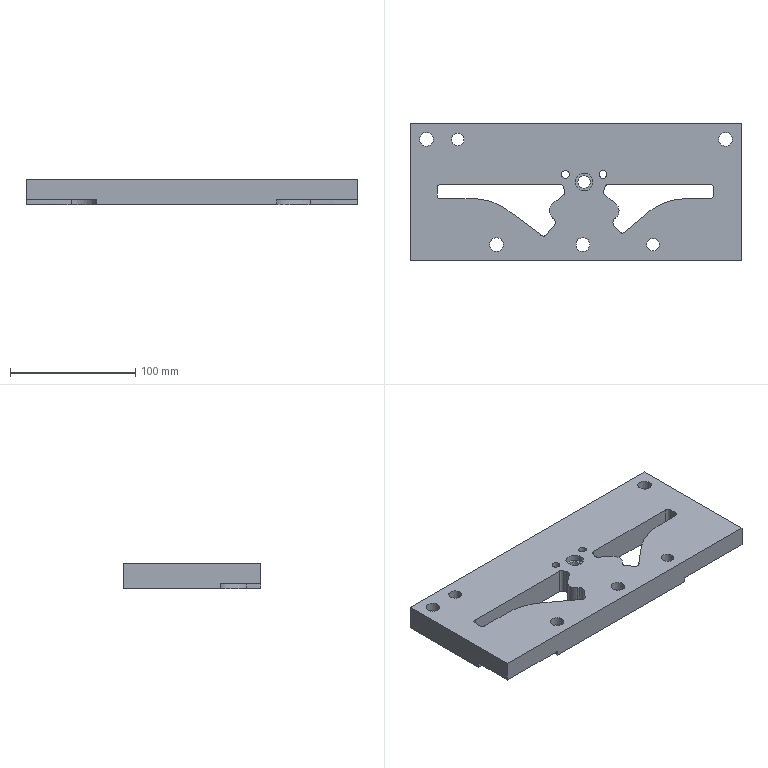Part | STEP file | 403_id1222_x_t | 1 solid | 92 faces | box 265 x 110 x 20 mm | volume 416142 mm3 | cylinder 41 | plane 37 | spline 14 | commonest cylinder face diameters 6 x10 11 x6 14 x5 17 x4 4 x3 10 x3